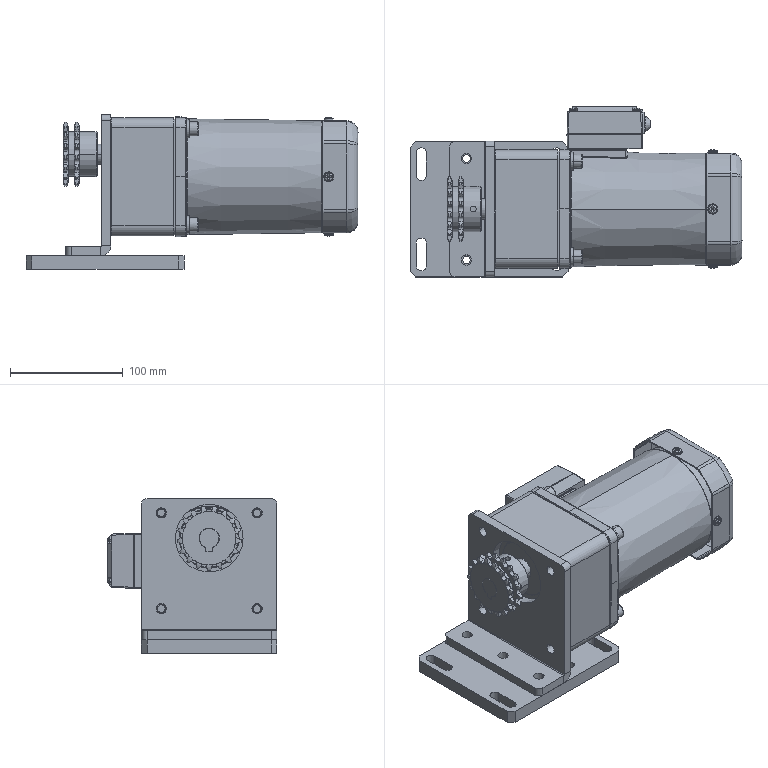Part | SolidWorks | 11 solids | 3132 faces | volume 1354603 mm3 | plane 1589 | cylinder 799 | spline 648 | cone 82 | torus 14 | commonest cylinder face diameters 2 x85 3 x59 4 x52 5.08 x46 8 x46 0.5 x44